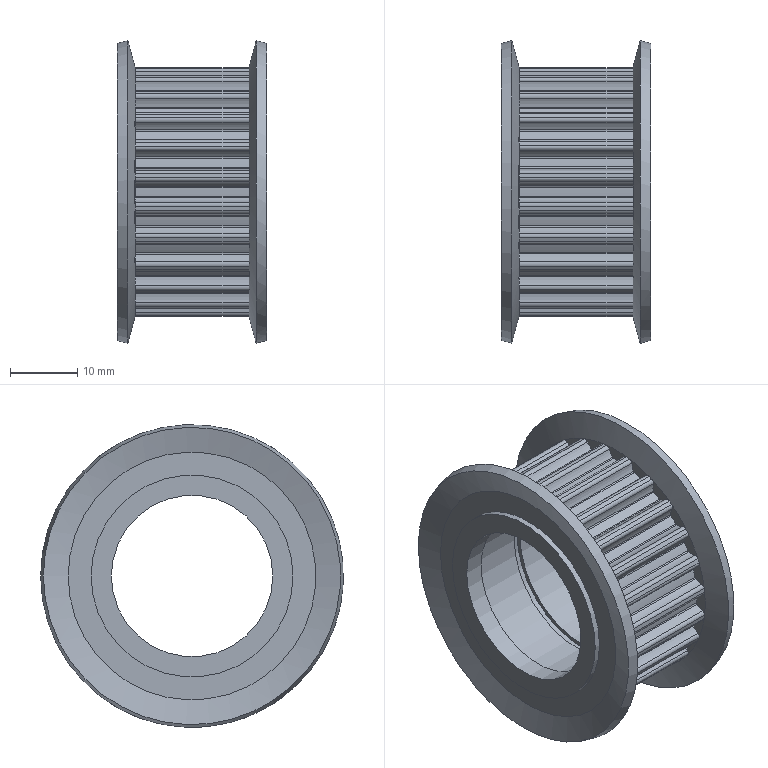Part | NX | features BODY_5003_016_C-AHTF24S5M150 2 | 1 solid | 238 faces | box 22.17 x 45 x 45 mm | volume 11397 mm3 | cylinder 199 | plane 33 | cone 6 | commonest cylinder face diameters 0.5 x48 1.1 x48 6.55 x48 33.7 x24 37.24 x24 26 x2